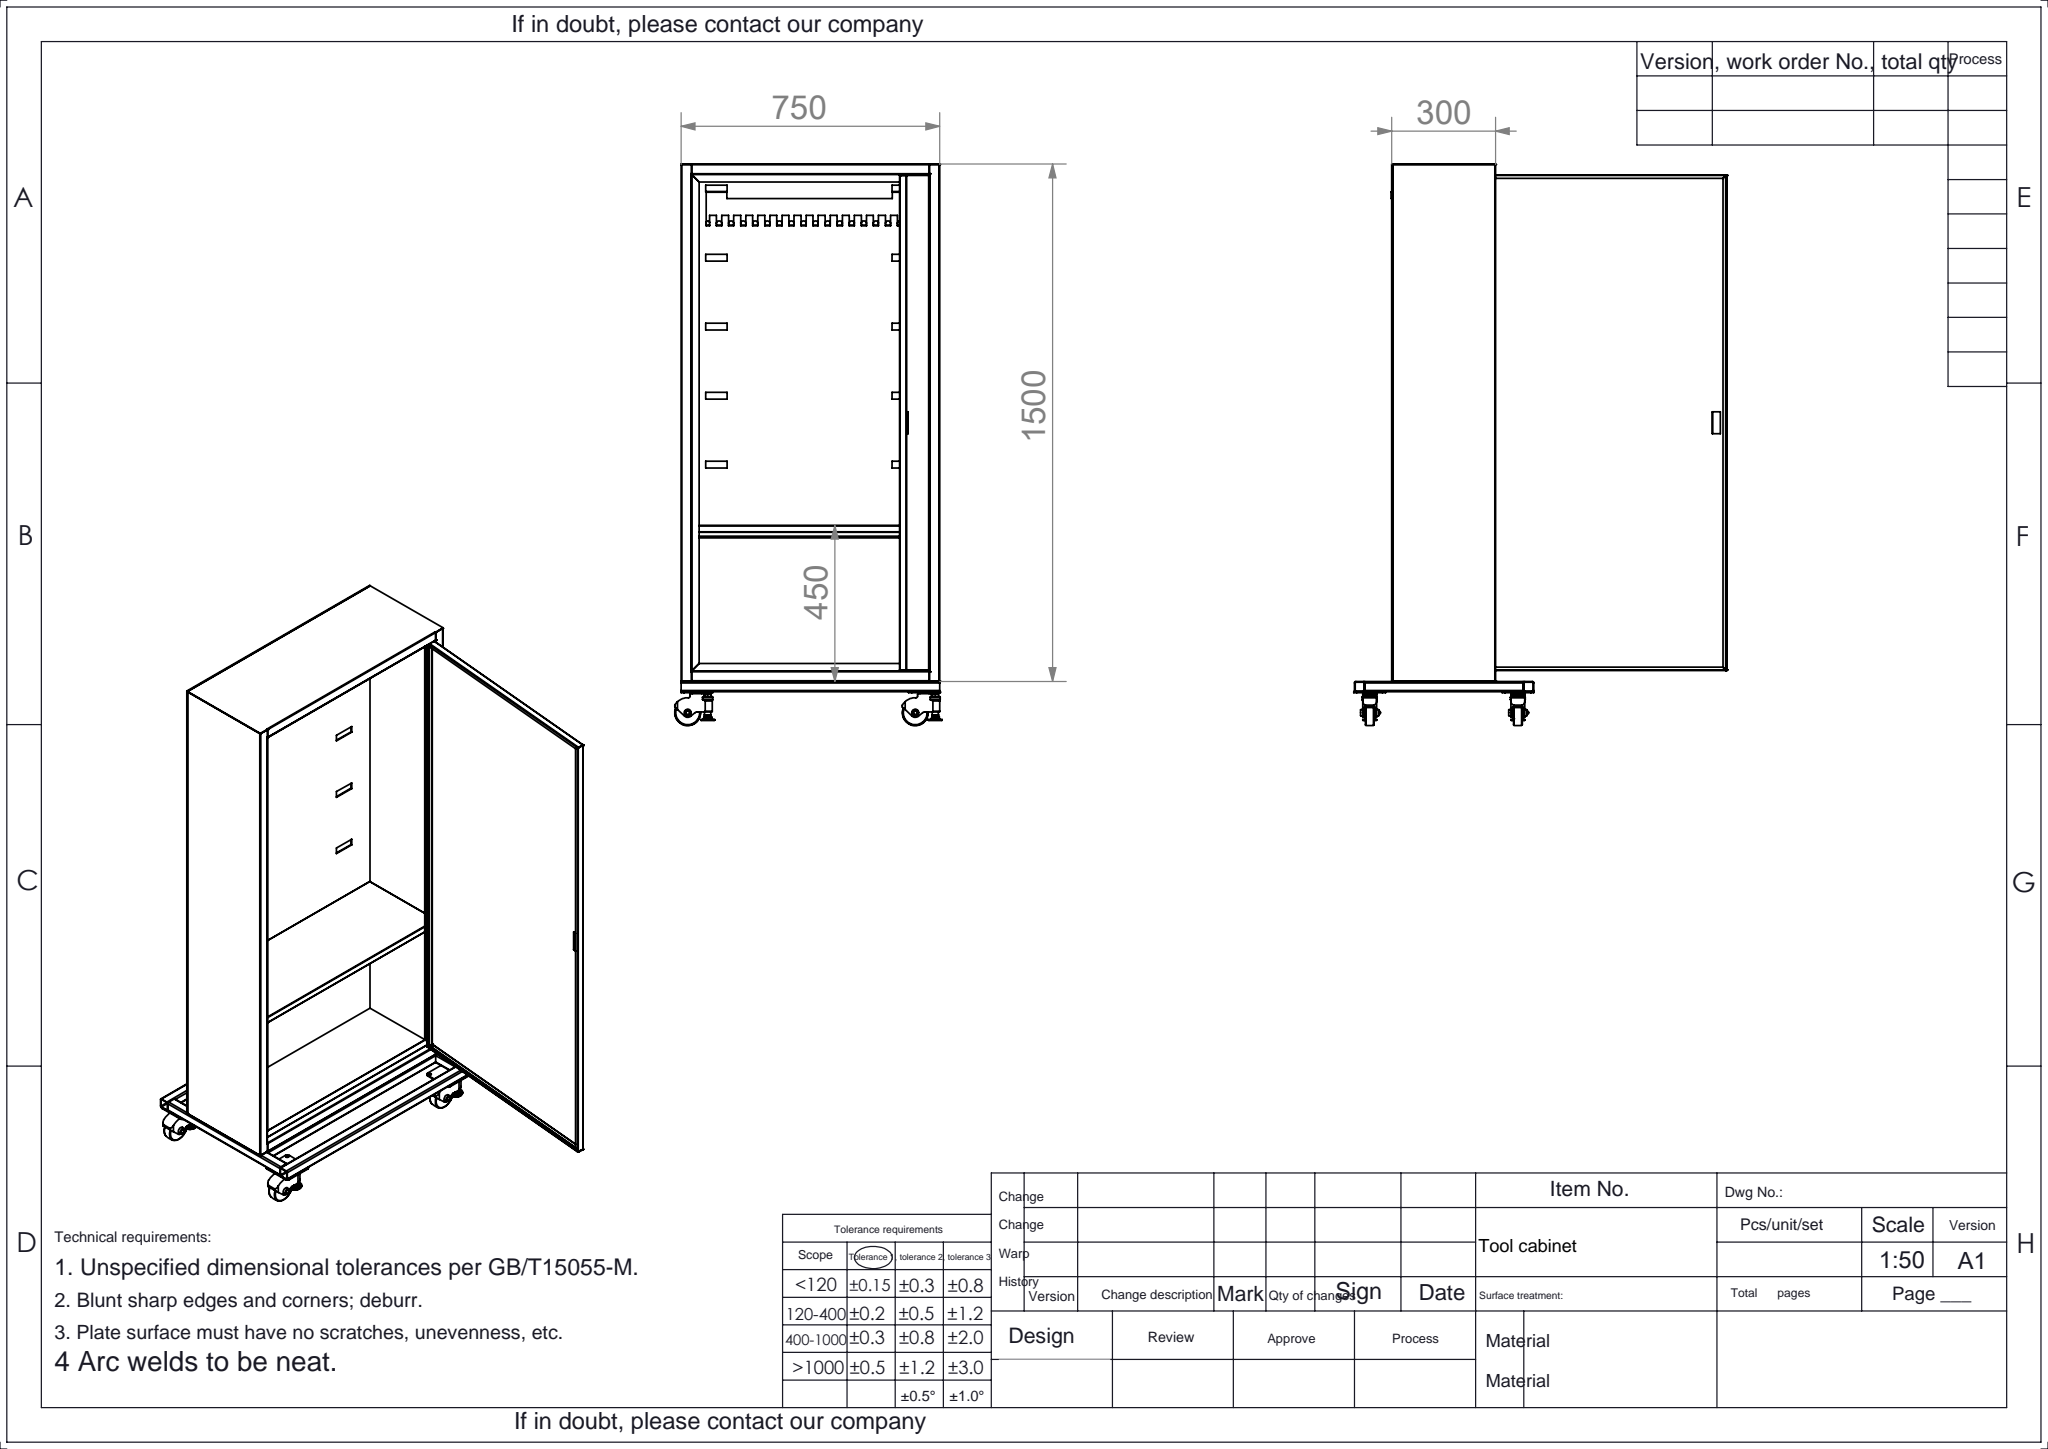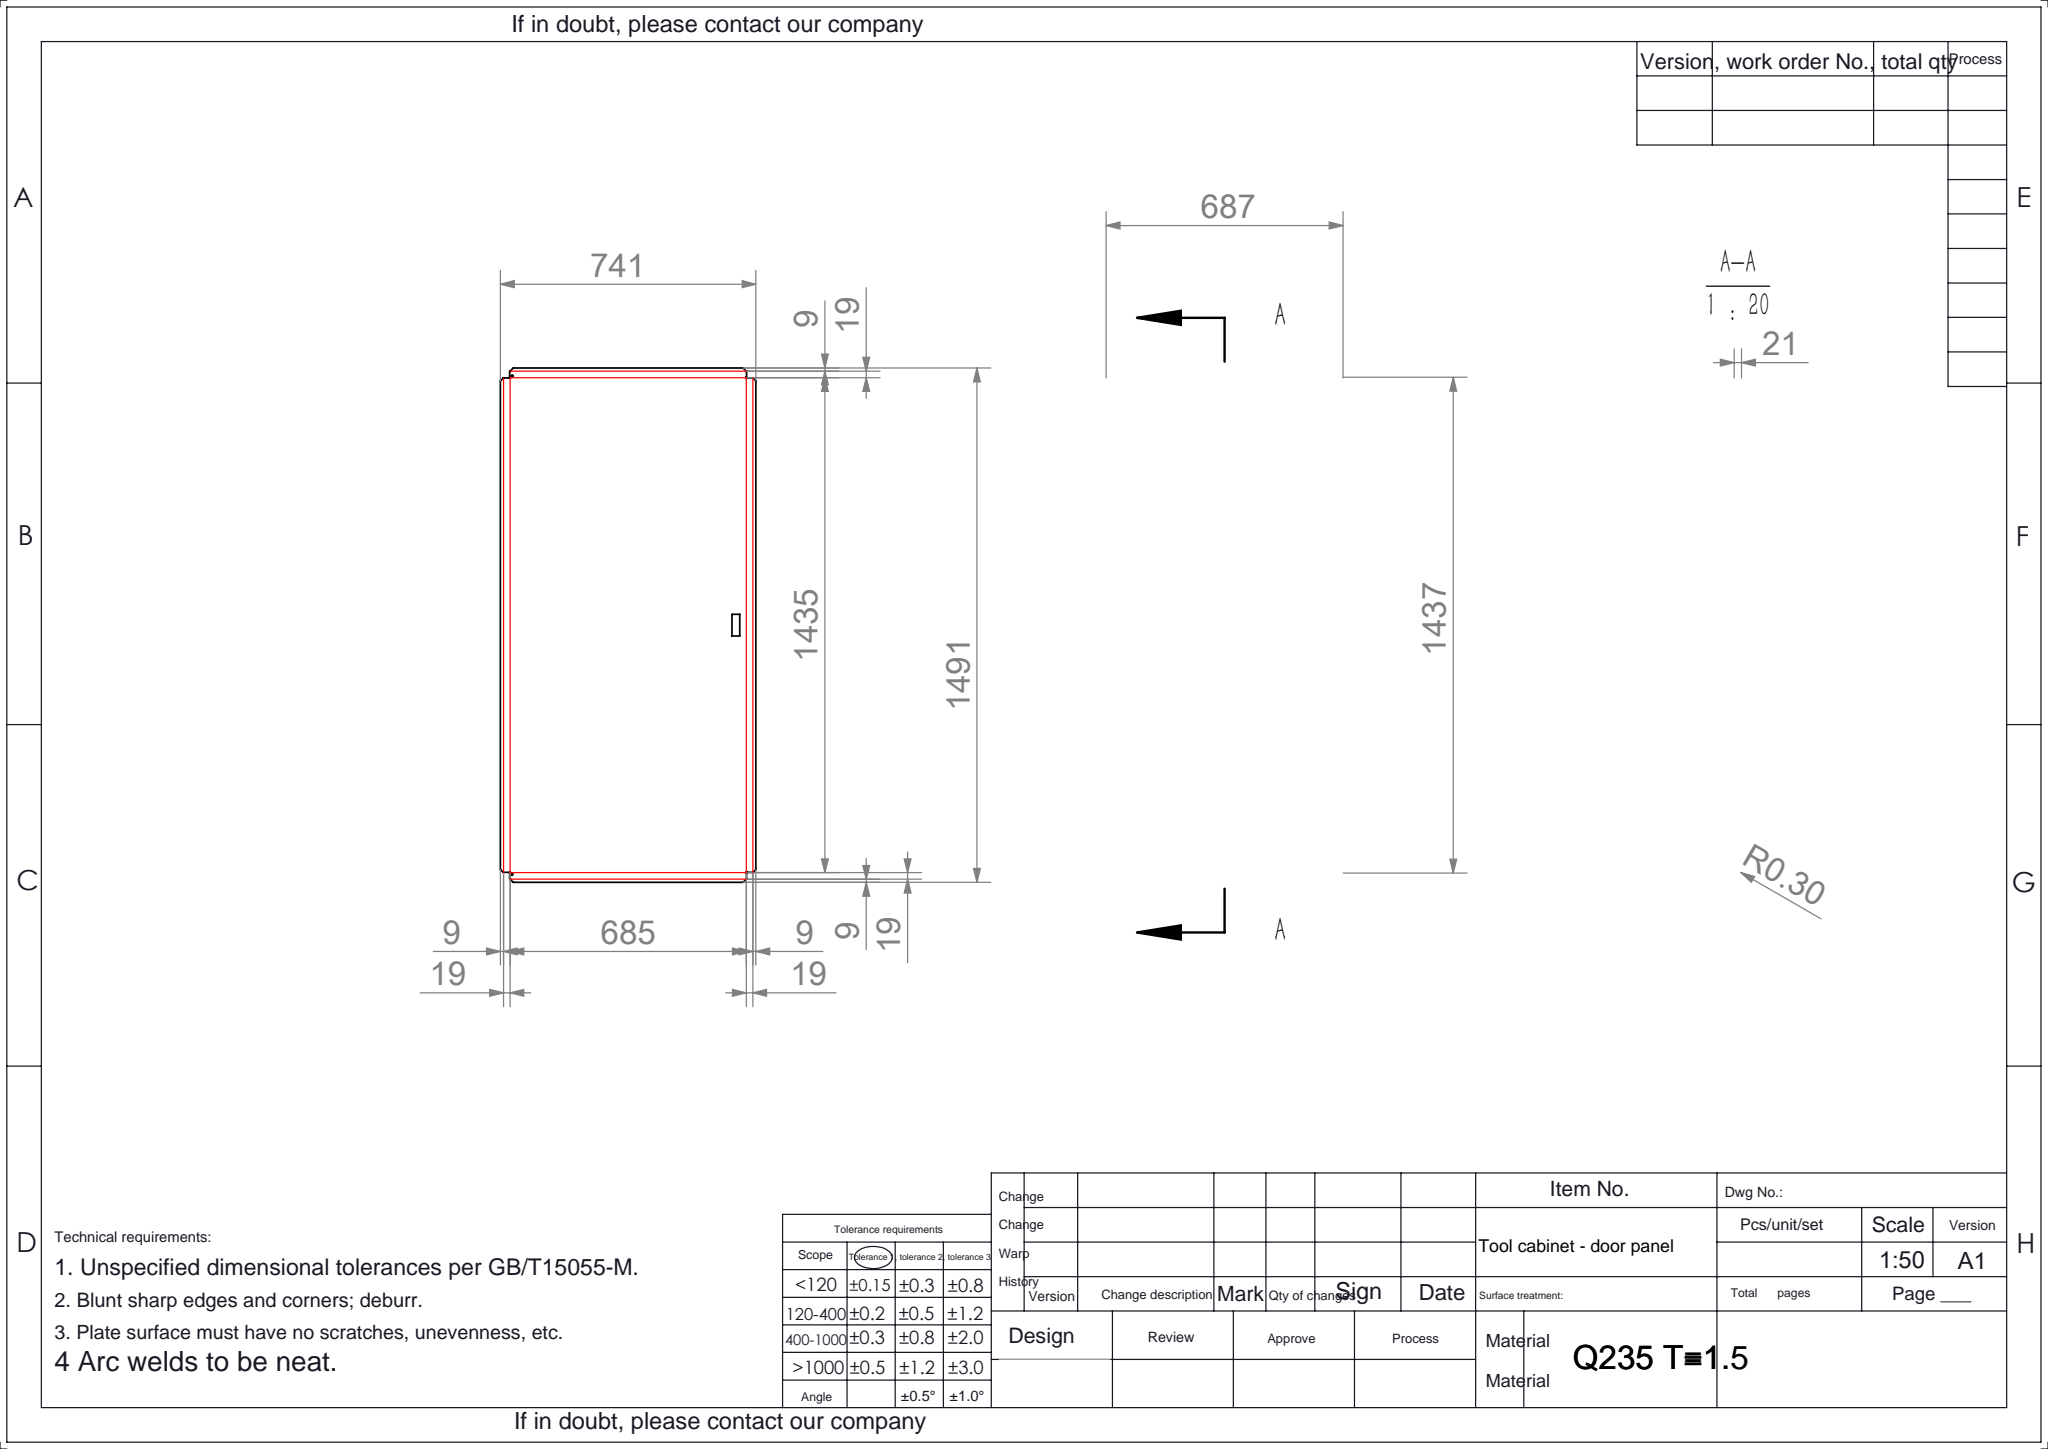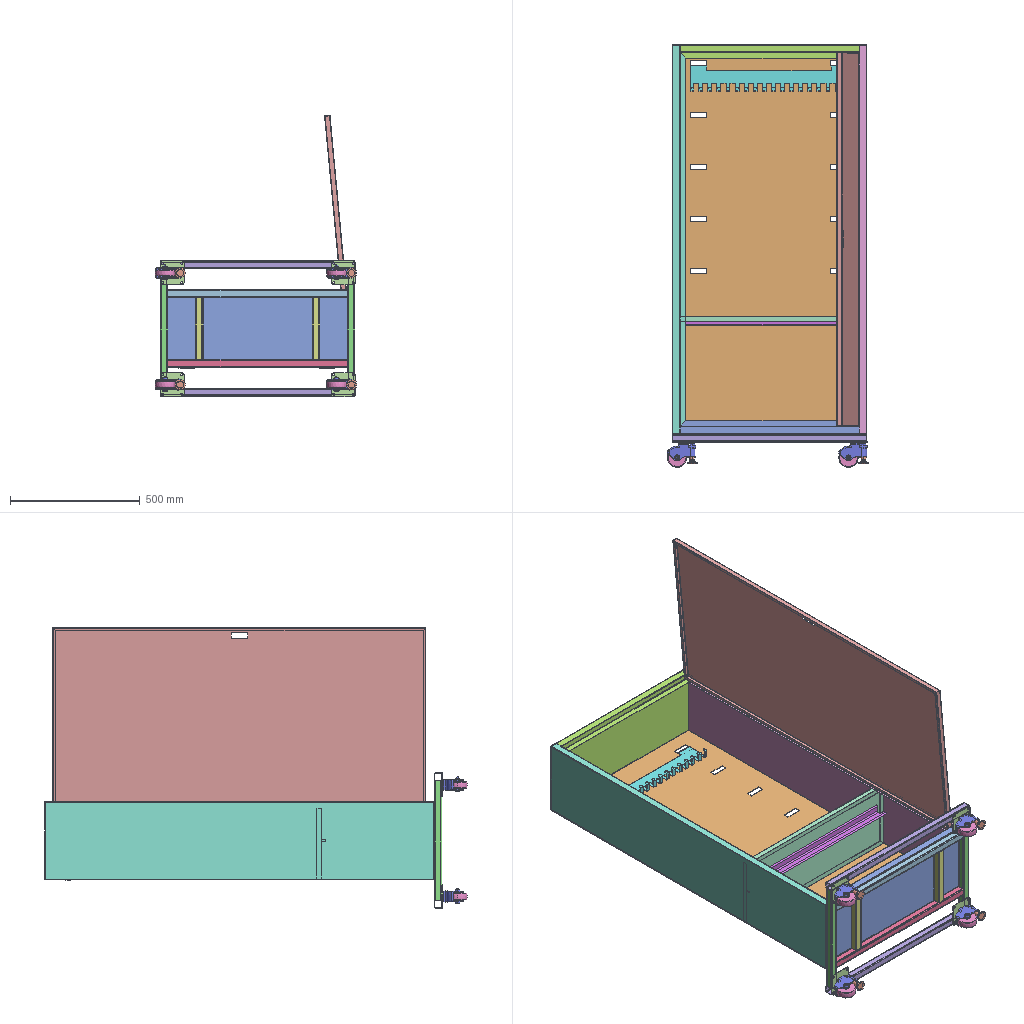Assembly | SolidWorks | 22 different items | 40 placed | box 775 x 1628 x 1082 mm
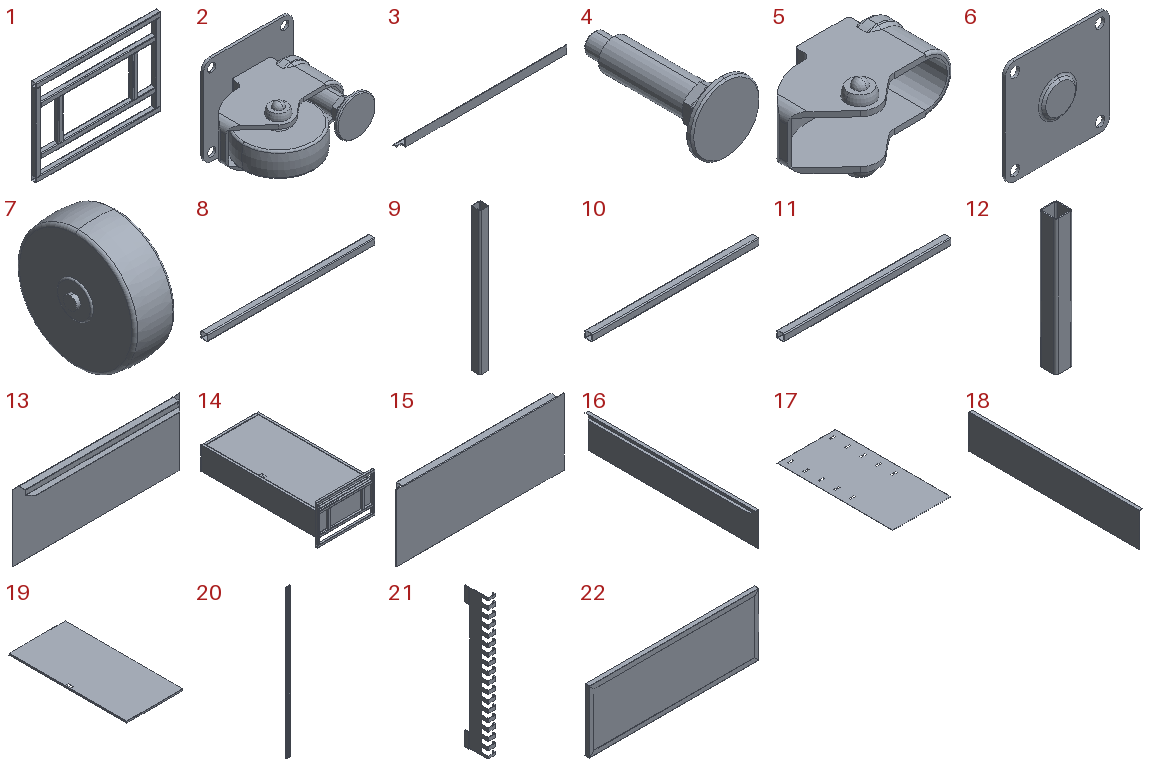Parts list (item | name | quantity | parent item | size | volume | features):
1 | (subassembly) | x1 | - | 750 x 30 x 520 mm | 913991 mm3 | -
2 | (subassembly) | x4 | - | 115.5 x 98 x 92 mm | 222779 mm3 | features AEMSimFeature 1
3 | - | x1 | - | 747 x 35 x 35 mm | 228267 mm3 | features Cut 1, WeldMemberFeat 1, WeldmentFeature 1
4 | - | x4 | in 2 | 40 x 77.4 x 40 mm | 22460 mm3 | features BaseBody 1
5 | - | x4 | in 2 | 110 x 68.7 x 58 mm | 68662 mm3 | features BaseBody 1
6 | - | x4 | in 2 | 92 x 5.3 x 92 mm | 22833 mm3 | features BaseBody 1
7 | - | x4 | in 2 | 32 x 75 x 75 mm | 108825 mm3 | features BaseBody 1
8 | - | x2 | in 1 | 750 x 30 x 30 mm | 160274 mm3 | features BaseBody 1
9 | - | x2 | in 1 | 30 x 30 x 460 mm | 98302 mm3 | features BaseBody 1
10 | - | x1 | in 1 | 690 x 30 x 30 mm | 147452 mm3 | features BaseBody 1, MoveFace 1
11 | - | x1 | in 1 | 690 x 30 x 30 mm | 147452 mm3 | features BaseBody 1
12 | - | x2 | in 1 | 30 x 30 x 238.5 mm | 50967 mm3 | features BaseBody 1
13 | - | x1 | - | 750 x 52 x 298.5 mm | 408654 mm3 | features BaseBody 1, FlatPattern 1, FlattenBends 1, ProcessBends 1, SheetMetal 1
14 | - | x1 | - | 750 x 1530 x 520 mm | 6723347 mm3 | features ICE 27, MoveFace 8, DelFace 7, FlatPattern 5, FlattenBends 5, ProcessBends 5, SheetMetal 5, CombineBodies 4, 3DProfileFeature 2, Extrusion 1, Fillet 1, LibraryFeature 1, Rip 1, Shell 1, Split 1, WeldMemberFeat 1, WeldmentFeature 1
15 | - | x1 | - | 750 x 52 x 298.5 mm | 408652 mm3 | features BaseBody 1, FlatPattern 1, FlattenBends 1, ProcessBends 1, SheetMetal 1
16 | - | x1 | - | 52 x 1497 x 298.5 mm | 825530 mm3 | features BaseBody 1, FlatPattern 1, FlattenBends 1, ProcessBends 1, SheetMetal 1
17 | - | x1 | - | 750 x 1500 x 2.5 mm | 2781500 mm3 | features Cut 1, FlatPattern 1, SMBaseFlange 1, SheetMetal 1
18 | - | x1 | - | 52 x 1497 x 298.5 mm | 825530 mm3 | features BaseBody 1, DelFace 1, FlatPattern 1, FlattenBends 1, ProcessBends 1, SheetMetal 1
19 | - | x1 | - | 687 x 1437 x 21 mm | 1650433 mm3 | features DelFace 3, BaseBody 1, FlatPattern 1, FlattenBends 1, ProcessBends 1, SheetMetal 1
20 | - | x1 | - | 40 x 6.5 x 1430 mm | 103752 mm3 | features FlatPattern 1, SMBaseFlange 1, SheetMetal 1
21 | - | x1 | - | 37.5 x 99 x 600 mm | 79648 mm3 | features ICE 4, LPattern 2, FlatPattern 1, MirrorPattern 1, SMBaseFlange 1, SheetMetal 1
22 | - | x1 | - | 745 x 20 x 273.8 mm | 278470 mm3 | features CornerFeat 1, FlatPattern 1, FlattenBends 1, ProcessBends 1, SheetMetal 1, SplitBody 1
Mates (type | each side: item.copy, entity, surface, feature):
Coincident | 16.1 face plane Imported1 | 17.1 face plane Base-Flange2
Coincident | 13.1 face plane Imported1 | 17.1 face plane Base-Flange2 | 2 times
Coincident | 15.1 face plane Imported1 | 11.1 face plane Imported1 | 2 times
Concentric | 19.1 face cylinder Imported6 | 13.1 face cylinder Imported1
DistanceDim | 13.1 face plane Imported1 | 19.1 face plane Imported6
Coincident | 16.1 face plane Imported1 | 9.1 face plane Imported1
LimitPlanarAngleDim | 19.1 face plane Imported6 | 18.1 face plane Imported1
Coincident | 19.1 face plane Imported6 | 20.1 face plane Base-Flange1
Width | 20.1 face plane Base-Flange1 | 20.1 face plane Base-Flange1 | 19.1 face plane Imported6 | 19.1 face plane Imported6
Width | 19.1 face plane Imported6 | 19.1 face plane Imported6 | 20.1 face plane Base-Flange1 | 20.1 face plane Base-Flange1
Width | 18.1 face plane Imported1 | 16.1 face plane Imported1 | 3.1 face plane Angle Iron 35 X 35 X 5(1) | 3.1 face plane Angle Iron 35 X 35 X 5(1)
Parallel | 15.1 face plane Imported1 | 3.1 face plane Angle Iron 35 X 35 X 5(1)
Width | 17.1 face plane Base-Flange2 | 18.1 face plane Imported1 | 3.1 face plane Angle Iron 35 X 35 X 5(1) | 3.1 face plane Angle Iron 35 X 35 X 5(1)
DistanceDim | 3.1 face plane Angle Iron 35 X 35 X 5(1) | 15.1 face plane Imported1
Width | 22.1 face plane Base Part-Tool Cabinet-1 | 22.1 face plane Base Part-Tool Cabinet-1 | 16.1 face plane Imported1 | 18.1 face plane Imported1
Coincident | 17.1 face plane Base-Flange2 | 22.1 face plane Base Part-Tool Cabinet-1
Coincident | 9.2 face plane Imported1 | 6.1 face plane CMJZ75-N-swivel(1)
Coincident | 8.1 face plane Imported1 | 6.1 face plane CMJZ75-N-swivel(1) | 2 times
Coincident | 17.1 face plane Base-Flange2 | 21.1 face plane Base-Flange1
Width | 21.1 face plane Base-Flange1 | 21.1 face plane Cut-Extrude1 | 17.1 face plane Cut-Extrude1 | 17.1 face plane Cut-Extrude1
Coincident | 17.1 face plane Cut-Extrude1 | 21.1 face plane Base-Flange1
Coincident | 3.1 face plane Angle Iron 35 X 35 X 5(1) | 22.1 face plane Base Part-Tool Cabinet-1